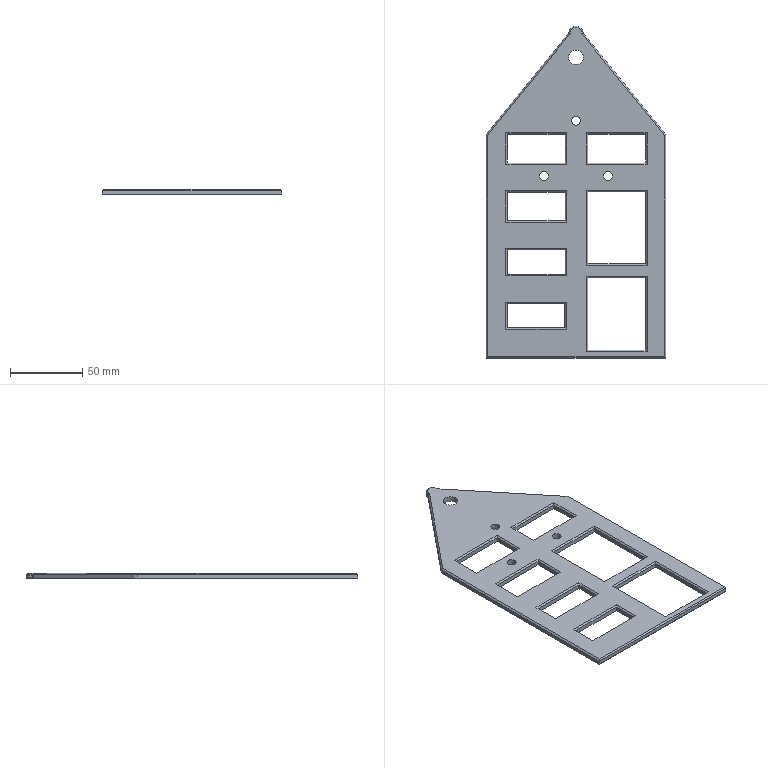Part | SolidWorks | features Chamfer 8, Fillet 2, Extrusion 1, ICE 1 | 1 solid | 110 faces | box 124.097 x 229.379 x 4 mm | volume 63027 mm3 | plane 75 | cylinder 17 | spline 12 | cone 4 | torus 2 | commonest cylinder face diameters 10 x8 6 x6 2 x2 9.895 x1